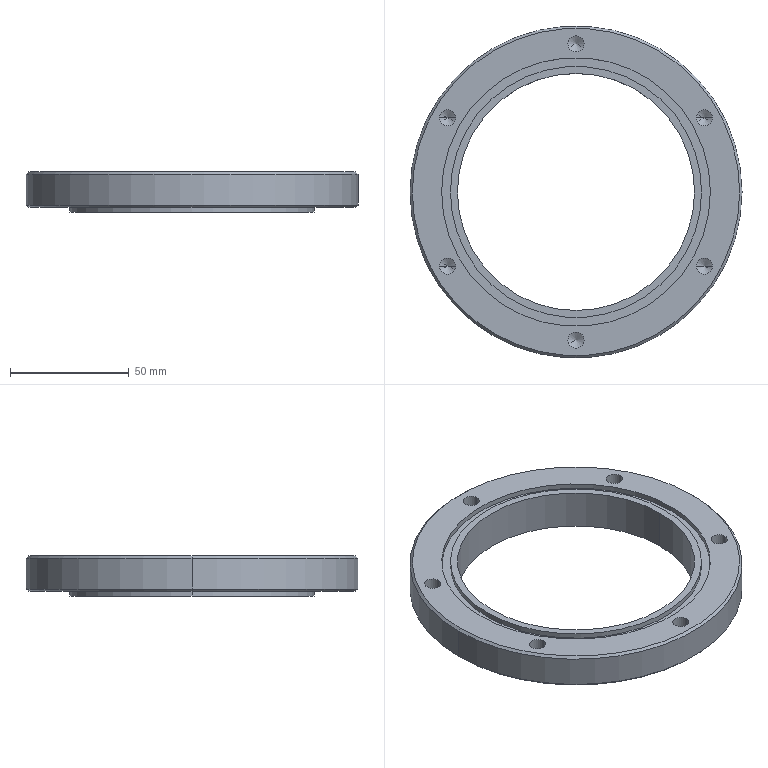Part | SolidWorks | features ICE 3, Chamfer 1, Extrusion 1, HoleWzd 1 | 1 solid | 43 faces | box 140 x 140 x 17 mm | volume 108486 mm3 | cylinder 22 | cone 16 | plane 5 | commonest cylinder face diameters 6.8 x12 100 x2 103 x2 105.9 x2 113.3 x2 140 x2
STEP:
#1=CARTESIAN_POINT('',(69.,0.,17.));
#2=VERTEX_POINT('',#1);
#3=CARTESIAN_POINT('',(-69.,0.,17.));
#4=VERTEX_POINT('',#3);
#5=CARTESIAN_POINT('',(0.,0.,17.));
#6=DIRECTION('',(0.,0.,1.));
#7=DIRECTION('',(1.,0.,0.));
#8=AXIS2_PLACEMENT_3D('',#5,#6,#7);
#9=CIRCLE('',#8,69.);
#10=EDGE_CURVE('',#2,#4,#9,.T.);
#11=ORIENTED_EDGE('',*,*,#10,.F.);
#12=CARTESIAN_POINT('',(70.,0.,16.));
#13=VERTEX_POINT('',#12);
#14=CARTESIAN_POINT('',(69.,0.,17.));
#15=DIRECTION('',(0.7071,0.,-0.7071));
#16=VECTOR('',#15,1000.);
#17=LINE('',#14,#16);
#18=EDGE_CURVE('',#2,#13,#17,.T.);
#19=ORIENTED_EDGE('',*,*,#18,.T.);
#20=CARTESIAN_POINT('',(-70.,0.,16.));
#21=VERTEX_POINT('',#20);
#22=CARTESIAN_POINT('',(0.,0.,16.));
#23=DIRECTION('',(0.,0.,-1.));
#24=DIRECTION('',(1.,0.,0.));
#25=AXIS2_PLACEMENT_3D('',#22,#23,#24);
#26=CIRCLE('',#25,70.);
#27=EDGE_CURVE('',#21,#13,#26,.T.);
#28=ORIENTED_EDGE('',*,*,#27,.F.);
#29=CARTESIAN_POINT('',(-69.,0.,17.));
#30=DIRECTION('',(-0.7071,0.,-0.7071));
#31=VECTOR('',#30,1000.);
#32=LINE('',#29,#31);
#33=EDGE_CURVE('',#4,#21,#32,.T.);
#34=ORIENTED_EDGE('',*,*,#33,.F.);
#35=EDGE_LOOP('',(#11,#19,#28,#34));
#36=FACE_OUTER_BOUND('',#35,.T.);
#37=CARTESIAN_POINT('',(0.,0.,17.));
#38=DIRECTION('',(0.,0.,-1.));
#39=DIRECTION('',(-1.,0.,0.));
#40=AXIS2_PLACEMENT_3D('',#37,#38,#39);
#41=CONICAL_SURFACE('',#40,69.,0.7854);
#42=ADVANCED_FACE('',(#36),#41,.T.);
#43=CARTESIAN_POINT('',(-69.,0.,2.));
#44=VERTEX_POINT('',#43);
#45=CARTESIAN_POINT('',(69.,0.,2.));
#46=VERTEX_POINT('',#45);
#47=CARTESIAN_POINT('',(0.,0.,2.));
#48=DIRECTION('',(0.,0.,-1.));
#49=DIRECTION('',(-1.,0.,0.));
#50=AXIS2_PLACEMENT_3D('',#47,#48,#49);
#51=CIRCLE('',#50,69.);
#52=EDGE_CURVE('',#44,#46,#51,.T.);
#53=ORIENTED_EDGE('',*,*,#52,.F.);
#54=CARTESIAN_POINT('',(-70.,0.,3.));
#55=VERTEX_POINT('',#54);
#56=CARTESIAN_POINT('',(-69.,0.,2.));
#57=DIRECTION('',(-0.7071,0.,0.7071));
#58=VECTOR('',#57,1000.);
#59=LINE('',#56,#58);
#60=EDGE_CURVE('',#44,#55,#59,.T.);
#61=ORIENTED_EDGE('',*,*,#60,.T.);
#62=CARTESIAN_POINT('',(70.,0.,3.));
#63=VERTEX_POINT('',#62);
#64=CARTESIAN_POINT('',(0.,0.,3.));
#65=DIRECTION('',(0.,0.,1.));
#66=DIRECTION('',(-1.,0.,0.));
#67=AXIS2_PLACEMENT_3D('',#64,#65,#66);
#68=CIRCLE('',#67,70.);
#69=EDGE_CURVE('',#63,#55,#68,.T.);
#70=ORIENTED_EDGE('',*,*,#69,.F.);
#71=CARTESIAN_POINT('',(69.,0.,2.));
#72=DIRECTION('',(0.7071,0.,0.7071));
#73=VECTOR('',#72,1000.);
#74=LINE('',#71,#73);
#75=EDGE_CURVE('',#46,#63,#74,.T.);
#76=ORIENTED_EDGE('',*,*,#75,.F.);
#77=EDGE_LOOP('',(#53,#61,#70,#76));
#78=FACE_OUTER_BOUND('',#77,.T.);
#79=CARTESIAN_POINT('',(0.,0.,2.));
#80=DIRECTION('',(0.,0.,1.));
#81=DIRECTION('',(1.,0.,0.));
#82=AXIS2_PLACEMENT_3D('',#79,#80,#81);
#83=CONICAL_SURFACE('',#82,69.,0.7854);
#84=ADVANCED_FACE('',(#78),#83,.T.);
#85=CARTESIAN_POINT('',(-3.4,62.5,7.));
#86=VERTEX_POINT('',#85);
#87=CARTESIAN_POINT('',(3.4,62.5,7.));
#88=VERTEX_POINT('',#87);
#89=CARTESIAN_POINT('',(0.,62.5,7.));
#90=DIRECTION('',(0.,0.,1.));
#91=DIRECTION('',(1.,0.,0.));
#92=AXIS2_PLACEMENT_3D('',#89,#90,#91);
#93=CIRCLE('',#92,3.4);
#94=EDGE_CURVE('',#86,#88,#93,.T.);
#95=ORIENTED_EDGE('',*,*,#94,.F.);
#96=CARTESIAN_POINT('',(-3.4,62.5,17.));
#97=VERTEX_POINT('',#96);
#98=CARTESIAN_POINT('',(-3.4,62.5,17.));
#99=DIRECTION('',(0.,0.,1.));
#100=VECTOR('',#99,1000.);
#101=LINE('',#98,#100);
#102=EDGE_CURVE('',#86,#97,#101,.T.);
#103=ORIENTED_EDGE('',*,*,#102,.T.);
#104=CARTESIAN_POINT('',(3.4,62.5,17.));
#105=VERTEX_POINT('',#104);
#106=CARTESIAN_POINT('',(0.,62.5,17.));
#107=DIRECTION('',(0.,0.,1.));
#108=DIRECTION('',(1.,0.,0.));
#109=AXIS2_PLACEMENT_3D('',#106,#107,#108);
#110=CIRCLE('',#109,3.4);
#111=EDGE_CURVE('',#97,#105,#110,.T.);
#112=ORIENTED_EDGE('',*,*,#111,.T.);
#113=CARTESIAN_POINT('',(3.4,62.5,17.));
#114=DIRECTION('',(0.,0.,1.));
#115=VECTOR('',#114,1000.);
#116=LINE('',#113,#115);
#117=EDGE_CURVE('',#88,#105,#116,.T.);
#118=ORIENTED_EDGE('',*,*,#117,.F.);
#119=EDGE_LOOP('',(#95,#103,#112,#118));
#120=FACE_OUTER_BOUND('',#119,.T.);
#121=CARTESIAN_POINT('',(0.,62.5,17.));
#122=DIRECTION('',(0.,0.,1.));
#123=DIRECTION('',(1.,0.,0.));
#124=AXIS2_PLACEMENT_3D('',#121,#122,#123);
#125=CYLINDRICAL_SURFACE('',#124,3.4);
#126=ADVANCED_FACE('',(#120),#125,.F.);
#127=CARTESIAN_POINT('',(0.,62.5,4.957));
#128=VERTEX_POINT('',#127);
#129=CARTESIAN_POINT('',(3.4,62.5,7.));
#130=DIRECTION('',(0.8572,0.,0.515));
#131=VECTOR('',#130,1000.);
#132=LINE('',#129,#131);
#133=EDGE_CURVE('',#128,#88,#132,.T.);
#134=ORIENTED_EDGE('',*,*,#133,.F.);
#135=CARTESIAN_POINT('',(-3.4,62.5,7.));
#136=DIRECTION('',(-0.8572,0.,0.515));
#137=VECTOR('',#136,1000.);
#138=LINE('',#135,#137);
#139=EDGE_CURVE('',#128,#86,#138,.T.);
#140=ORIENTED_EDGE('',*,*,#139,.T.);
#141=ORIENTED_EDGE('',*,*,#94,.T.);
#142=EDGE_LOOP('',(#134,#140,#141));
#143=FACE_OUTER_BOUND('',#142,.T.);
#144=CARTESIAN_POINT('',(0.,62.5,7.));
#145=DIRECTION('',(0.,0.,1.));
#146=DIRECTION('',(1.,0.,0.));
#147=AXIS2_PLACEMENT_3D('',#144,#145,#146);
#148=CONICAL_SURFACE('',#147,3.4,1.03);
#149=ADVANCED_FACE('',(#143),#148,.F.);
#150=CARTESIAN_POINT('',(50.727,31.25,7.));
#151=VERTEX_POINT('',#150);
#152=CARTESIAN_POINT('',(57.527,31.25,7.));
#153=VERTEX_POINT('',#152);
#154=CARTESIAN_POINT('',(54.127,31.25,7.));
#155=DIRECTION('',(0.,0.,1.));
#156=DIRECTION('',(1.,0.,0.));
#157=AXIS2_PLACEMENT_3D('',#154,#155,#156);
#158=CIRCLE('',#157,3.4);
#159=EDGE_CURVE('',#151,#153,#158,.T.);
#160=ORIENTED_EDGE('',*,*,#159,.F.);
#161=CARTESIAN_POINT('',(50.727,31.25,17.));
#162=VERTEX_POINT('',#161);
#163=CARTESIAN_POINT('',(50.727,31.25,17.));
#164=DIRECTION('',(0.,0.,1.));
#165=VECTOR('',#164,1000.);
#166=LINE('',#163,#165);
#167=EDGE_CURVE('',#151,#162,#166,.T.);
#168=ORIENTED_EDGE('',*,*,#167,.T.);
#169=CARTESIAN_POINT('',(57.527,31.25,17.));
#170=VERTEX_POINT('',#169);
#171=CARTESIAN_POINT('',(54.127,31.25,17.));
#172=DIRECTION('',(0.,0.,1.));
#173=DIRECTION('',(1.,0.,0.));
#174=AXIS2_PLACEMENT_3D('',#171,#172,#173);
#175=CIRCLE('',#174,3.4);
#176=EDGE_CURVE('',#162,#170,#175,.T.);
#177=ORIENTED_EDGE('',*,*,#176,.T.);
#178=CARTESIAN_POINT('',(57.527,31.25,17.));
#179=DIRECTION('',(0.,0.,1.));
#180=VECTOR('',#179,1000.);
#181=LINE('',#178,#180);
#182=EDGE_CURVE('',#153,#170,#181,.T.);
#183=ORIENTED_EDGE('',*,*,#182,.F.);
#184=EDGE_LOOP('',(#160,#168,#177,#183));
#185=FACE_OUTER_BOUND('',#184,.T.);
#186=CARTESIAN_POINT('',(54.127,31.25,17.));
#187=DIRECTION('',(0.,0.,1.));
#188=DIRECTION('',(1.,0.,0.));
#189=AXIS2_PLACEMENT_3D('',#186,#187,#188);
#190=CYLINDRICAL_SURFACE('',#189,3.4);
#191=ADVANCED_FACE('',(#185),#190,.F.);
#192=CARTESIAN_POINT('',(54.127,31.25,4.957));
#193=VERTEX_POINT('',#192);
#194=CARTESIAN_POINT('',(57.527,31.25,7.));
#195=DIRECTION('',(0.8572,0.,0.515));
#196=VECTOR('',#195,1000.);
#197=LINE('',#194,#196);
#198=EDGE_CURVE('',#193,#153,#197,.T.);
#199=ORIENTED_EDGE('',*,*,#198,.F.);
#200=CARTESIAN_POINT('',(50.727,31.25,7.));
#201=DIRECTION('',(-0.8572,0.,0.515));
#202=VECTOR('',#201,1000.);
#203=LINE('',#200,#202);
#204=EDGE_CURVE('',#193,#151,#203,.T.);
#205=ORIENTED_EDGE('',*,*,#204,.T.);
#206=ORIENTED_EDGE('',*,*,#159,.T.);
#207=EDGE_LOOP('',(#199,#205,#206));
#208=FACE_OUTER_BOUND('',#207,.T.);
#209=CARTESIAN_POINT('',(54.127,31.25,7.));
#210=DIRECTION('',(0.,0.,1.));
#211=DIRECTION('',(1.,0.,0.));
#212=AXIS2_PLACEMENT_3D('',#209,#210,#211);
#213=CONICAL_SURFACE('',#212,3.4,1.03);
#214=ADVANCED_FACE('',(#208),#213,.F.);
#215=CARTESIAN_POINT('',(50.727,-31.25,7.));
#216=VERTEX_POINT('',#215);
#217=CARTESIAN_POINT('',(57.527,-31.25,7.));
#218=VERTEX_POINT('',#217);
#219=CARTESIAN_POINT('',(54.127,-31.25,7.));
#220=DIRECTION('',(0.,0.,1.));
#221=DIRECTION('',(1.,0.,0.));
#222=AXIS2_PLACEMENT_3D('',#219,#220,#221);
#223=CIRCLE('',#222,3.4);
#224=EDGE_CURVE('',#216,#218,#223,.T.);
#225=ORIENTED_EDGE('',*,*,#224,.F.);
#226=CARTESIAN_POINT('',(50.727,-31.25,17.));
#227=VERTEX_POINT('',#226);
#228=CARTESIAN_POINT('',(50.727,-31.25,17.));
#229=DIRECTION('',(0.,0.,1.));
#230=VECTOR('',#229,1000.);
#231=LINE('',#228,#230);
#232=EDGE_CURVE('',#216,#227,#231,.T.);
#233=ORIENTED_EDGE('',*,*,#232,.T.);
#234=CARTESIAN_POINT('',(57.527,-31.25,17.));
#235=VERTEX_POINT('',#234);
#236=CARTESIAN_POINT('',(54.127,-31.25,17.));
#237=DIRECTION('',(0.,0.,1.));
#238=DIRECTION('',(1.,0.,0.));
#239=AXIS2_PLACEMENT_3D('',#236,#237,#238);
#240=CIRCLE('',#239,3.4);
#241=EDGE_CURVE('',#227,#235,#240,.T.);
#242=ORIENTED_EDGE('',*,*,#241,.T.);
#243=CARTESIAN_POINT('',(57.527,-31.25,17.));
#244=DIRECTION('',(0.,0.,1.));
#245=VECTOR('',#244,1000.);
#246=LINE('',#243,#245);
#247=EDGE_CURVE('',#218,#235,#246,.T.);
#248=ORIENTED_EDGE('',*,*,#247,.F.);
#249=EDGE_LOOP('',(#225,#233,#242,#248));
#250=FACE_OUTER_BOUND('',#249,.T.);
#251=CARTESIAN_POINT('',(54.127,-31.25,17.));
#252=DIRECTION('',(0.,0.,1.));
#253=DIRECTION('',(1.,0.,0.));
#254=AXIS2_PLACEMENT_3D('',#251,#252,#253);
#255=CYLINDRICAL_SURFACE('',#254,3.4);
#256=ADVANCED_FACE('',(#250),#255,.F.);
#257=CARTESIAN_POINT('',(54.127,-31.25,4.957));
#258=VERTEX_POINT('',#257);
#259=CARTESIAN_POINT('',(57.527,-31.25,7.));
#260=DIRECTION('',(0.8572,0.,0.515));
#261=VECTOR('',#260,1000.);
#262=LINE('',#259,#261);
#263=EDGE_CURVE('',#258,#218,#262,.T.);
#264=ORIENTED_EDGE('',*,*,#263,.F.);
#265=CARTESIAN_POINT('',(50.727,-31.25,7.));
#266=DIRECTION('',(-0.8572,0.,0.515));
#267=VECTOR('',#266,1000.);
#268=LINE('',#265,#267);
#269=EDGE_CURVE('',#258,#216,#268,.T.);
#270=ORIENTED_EDGE('',*,*,#269,.T.);
#271=ORIENTED_EDGE('',*,*,#224,.T.);
#272=EDGE_LOOP('',(#264,#270,#271));
#273=FACE_OUTER_BOUND('',#272,.T.);
#274=CARTESIAN_POINT('',(54.127,-31.25,7.));
#275=DIRECTION('',(0.,0.,1.));
#276=DIRECTION('',(1.,0.,0.));
#277=AXIS2_PLACEMENT_3D('',#274,#275,#276);
#278=CONICAL_SURFACE('',#277,3.4,1.03);
#279=ADVANCED_FACE('',(#273),#278,.F.);
#280=CARTESIAN_POINT('',(-3.4,-62.5,7.));
#281=VERTEX_POINT('',#280);
#282=CARTESIAN_POINT('',(3.4,-62.5,7.));
#283=VERTEX_POINT('',#282);
#284=CARTESIAN_POINT('',(0.,-62.5,7.));
#285=DIRECTION('',(0.,0.,1.));
#286=DIRECTION('',(1.,0.,0.));
#287=AXIS2_PLACEMENT_3D('',#284,#285,#286);
#288=CIRCLE('',#287,3.4);
#289=EDGE_CURVE('',#281,#283,#288,.T.);
#290=ORIENTED_EDGE('',*,*,#289,.F.);
#291=CARTESIAN_POINT('',(-3.4,-62.5,17.));
#292=VERTEX_POINT('',#291);
#293=CARTESIAN_POINT('',(-3.4,-62.5,17.));
#294=DIRECTION('',(0.,0.,1.));
#295=VECTOR('',#294,1000.);
#296=LINE('',#293,#295);
#297=EDGE_CURVE('',#281,#292,#296,.T.);
#298=ORIENTED_EDGE('',*,*,#297,.T.);
#299=CARTESIAN_POINT('',(3.4,-62.5,17.));
#300=VERTEX_POINT('',#299);
#301=CARTESIAN_POINT('',(0.,-62.5,17.));
#302=DIRECTION('',(0.,0.,1.));
#303=DIRECTION('',(1.,0.,0.));
#304=AXIS2_PLACEMENT_3D('',#301,#302,#303);
#305=CIRCLE('',#304,3.4);
#306=EDGE_CURVE('',#292,#300,#305,.T.);
#307=ORIENTED_EDGE('',*,*,#306,.T.);
#308=CARTESIAN_POINT('',(3.4,-62.5,17.));
#309=DIRECTION('',(0.,0.,1.));
#310=VECTOR('',#309,1000.);
#311=LINE('',#308,#310);
#312=EDGE_CURVE('',#283,#300,#311,.T.);
#313=ORIENTED_EDGE('',*,*,#312,.F.);
#314=EDGE_LOOP('',(#290,#298,#307,#313));
#315=FACE_OUTER_BOUND('',#314,.T.);
#316=CARTESIAN_POINT('',(0.,-62.5,17.));
#317=DIRECTION('',(0.,0.,1.));
#318=DIRECTION('',(1.,0.,0.));
#319=AXIS2_PLACEMENT_3D('',#316,#317,#318);
#320=CYLINDRICAL_SURFACE('',#319,3.4);
#321=ADVANCED_FACE('',(#315),#320,.F.);
#322=CARTESIAN_POINT('',(0.,-62.5,4.957));
#323=VERTEX_POINT('',#322);
#324=CARTESIAN_POINT('',(3.4,-62.5,7.));
#325=DIRECTION('',(0.8572,0.,0.515));
#326=VECTOR('',#325,1000.);
#327=LINE('',#324,#326);
#328=EDGE_CURVE('',#323,#283,#327,.T.);
#329=ORIENTED_EDGE('',*,*,#328,.F.);
#330=CARTESIAN_POINT('',(-3.4,-62.5,7.));
#331=DIRECTION('',(-0.8572,0.,0.515));
#332=VECTOR('',#331,1000.);
#333=LINE('',#330,#332);
#334=EDGE_CURVE('',#323,#281,#333,.T.);
#335=ORIENTED_EDGE('',*,*,#334,.T.);
#336=ORIENTED_EDGE('',*,*,#289,.T.);
#337=EDGE_LOOP('',(#329,#335,#336));
#338=FACE_OUTER_BOUND('',#337,.T.);
#339=CARTESIAN_POINT('',(0.,-62.5,7.));
#340=DIRECTION('',(0.,0.,1.));
#341=DIRECTION('',(1.,0.,0.));
#342=AXIS2_PLACEMENT_3D('',#339,#340,#341);
#343=CONICAL_SURFACE('',#342,3.4,1.03);
#344=ADVANCED_FACE('',(#338),#343,.F.);
#345=CARTESIAN_POINT('',(-57.527,-31.25,7.));
#346=VERTEX_POINT('',#345);
#347=CARTESIAN_POINT('',(-50.727,-31.25,7.));
#348=VERTEX_POINT('',#347);
#349=CARTESIAN_POINT('',(-54.127,-31.25,7.));
#350=DIRECTION('',(0.,0.,1.));
#351=DIRECTION('',(1.,0.,0.));
#352=AXIS2_PLACEMENT_3D('',#349,#350,#351);
#353=CIRCLE('',#352,3.4);
#354=EDGE_CURVE('',#346,#348,#353,.T.);
#355=ORIENTED_EDGE('',*,*,#354,.F.);
#356=CARTESIAN_POINT('',(-57.527,-31.25,17.));
#357=VERTEX_POINT('',#356);
#358=CARTESIAN_POINT('',(-57.527,-31.25,17.));
#359=DIRECTION('',(0.,0.,1.));
#360=VECTOR('',#359,1000.);
#361=LINE('',#358,#360);
#362=EDGE_CURVE('',#346,#357,#361,.T.);
#363=ORIENTED_EDGE('',*,*,#362,.T.);
#364=CARTESIAN_POINT('',(-50.727,-31.25,17.));
#365=VERTEX_POINT('',#364);
#366=CARTESIAN_POINT('',(-54.127,-31.25,17.));
#367=DIRECTION('',(0.,0.,1.));
#368=DIRECTION('',(1.,0.,0.));
#369=AXIS2_PLACEMENT_3D('',#366,#367,#368);
#370=CIRCLE('',#369,3.4);
#371=EDGE_CURVE('',#357,#365,#370,.T.);
#372=ORIENTED_EDGE('',*,*,#371,.T.);
#373=CARTESIAN_POINT('',(-50.727,-31.25,17.));
#374=DIRECTION('',(0.,0.,1.));
#375=VECTOR('',#374,1000.);
#376=LINE('',#373,#375);
#377=EDGE_CURVE('',#348,#365,#376,.T.);
#378=ORIENTED_EDGE('',*,*,#377,.F.);
#379=EDGE_LOOP('',(#355,#363,#372,#378));
#380=FACE_OUTER_BOUND('',#379,.T.);
#381=CARTESIAN_POINT('',(-54.127,-31.25,17.));
#382=DIRECTION('',(0.,0.,1.));
#383=DIRECTION('',(1.,0.,0.));
#384=AXIS2_PLACEMENT_3D('',#381,#382,#383);
#385=CYLINDRICAL_SURFACE('',#384,3.4);
#386=ADVANCED_FACE('',(#380),#385,.F.);
#387=CARTESIAN_POINT('',(-54.127,-31.25,4.957));
#388=VERTEX_POINT('',#387);
#389=CARTESIAN_POINT('',(-50.727,-31.25,7.));
#390=DIRECTION('',(0.8572,0.,0.515));
#391=VECTOR('',#390,1000.);
#392=LINE('',#389,#391);
#393=EDGE_CURVE('',#388,#348,#392,.T.);
#394=ORIENTED_EDGE('',*,*,#393,.F.);
#395=CARTESIAN_POINT('',(-57.527,-31.25,7.));
#396=DIRECTION('',(-0.8572,0.,0.515));
#397=VECTOR('',#396,1000.);
#398=LINE('',#395,#397);
#399=EDGE_CURVE('',#388,#346,#398,.T.);
#400=ORIENTED_EDGE('',*,*,#399,.T.);
#401=ORIENTED_EDGE('',*,*,#354,.T.);
#402=EDGE_LOOP('',(#394,#400,#401));
#403=FACE_OUTER_BOUND('',#402,.T.);
#404=CARTESIAN_POINT('',(-54.127,-31.25,7.));
#405=DIRECTION('',(0.,0.,1.));
#406=DIRECTION('',(1.,0.,0.));
#407=AXIS2_PLACEMENT_3D('',#404,#405,#406);
#408=CONICAL_SURFACE('',#407,3.4,1.03);
#409=ADVANCED_FACE('',(#403),#408,.F.);
#410=CARTESIAN_POINT('',(-57.527,31.25,7.));
#411=VERTEX_POINT('',#410);
#412=CARTESIAN_POINT('',(-50.727,31.25,7.));
#413=VERTEX_POINT('',#412);
#414=CARTESIAN_POINT('',(-54.127,31.25,7.));
#415=DIRECTION('',(0.,0.,1.));
#416=DIRECTION('',(1.,0.,0.));
#417=AXIS2_PLACEMENT_3D('',#414,#415,#416);
#418=CIRCLE('',#417,3.4);
#419=EDGE_CURVE('',#411,#413,#418,.T.);
#420=ORIENTED_EDGE('',*,*,#419,.F.);
#421=CARTESIAN_POINT('',(-57.527,31.25,17.));
#422=VERTEX_POINT('',#421);
#423=CARTESIAN_POINT('',(-57.527,31.25,17.));
#424=DIRECTION('',(0.,0.,1.));
#425=VECTOR('',#424,1000.);
#426=LINE('',#423,#425);
#427=EDGE_CURVE('',#411,#422,#426,.T.);
#428=ORIENTED_EDGE('',*,*,#427,.T.);
#429=CARTESIAN_POINT('',(-50.727,31.25,17.));
#430=VERTEX_POINT('',#429);
#431=CARTESIAN_POINT('',(-54.127,31.25,17.));
#432=DIRECTION('',(0.,0.,1.));
#433=DIRECTION('',(1.,0.,0.));
#434=AXIS2_PLACEMENT_3D('',#431,#432,#433);
#435=CIRCLE('',#434,3.4);
#436=EDGE_CURVE('',#422,#430,#435,.T.);
#437=ORIENTED_EDGE('',*,*,#436,.T.);
#438=CARTESIAN_POINT('',(-50.727,31.25,17.));
#439=DIRECTION('',(0.,0.,1.));
#440=VECTOR('',#439,1000.);
#441=LINE('',#438,#440);
#442=EDGE_CURVE('',#413,#430,#441,.T.);
#443=ORIENTED_EDGE('',*,*,#442,.F.);
#444=EDGE_LOOP('',(#420,#428,#437,#443));
#445=FACE_OUTER_BOUND('',#444,.T.);
#446=CARTESIAN_POINT('',(-54.127,31.25,17.));
#447=DIRECTION('',(0.,0.,1.));
#448=DIRECTION('',(1.,0.,0.));
#449=AXIS2_PLACEMENT_3D('',#446,#447,#448);
#450=CYLINDRICAL_SURFACE('',#449,3.4);
#451=ADVANCED_FACE('',(#445),#450,.F.);
#452=CARTESIAN_POINT('',(-54.127,31.25,4.957));
#453=VERTEX_POINT('',#452);
#454=CARTESIAN_POINT('',(-50.727,31.25,7.));
#455=DIRECTION('',(0.8572,0.,0.515));
#456=VECTOR('',#455,1000.);
#457=LINE('',#454,#456);
#458=EDGE_CURVE('',#453,#413,#457,.T.);
#459=ORIENTED_EDGE('',*,*,#458,.F.);
#460=CARTESIAN_POINT('',(-57.527,31.25,7.));
#461=DIRECTION('',(-0.8572,0.,0.515));
#462=VECTOR('',#461,1000.);
#463=LINE('',#460,#462);
#464=EDGE_CURVE('',#453,#411,#463,.T.);
#465=ORIENTED_EDGE('',*,*,#464,.T.);
#466=ORIENTED_EDGE('',*,*,#419,.T.);
#467=EDGE_LOOP('',(#459,#465,#466));
#468=FACE_OUTER_BOUND('',#467,.T.);
#469=CARTESIAN_POINT('',(-54.127,31.25,7.));
#470=DIRECTION('',(0.,0.,1.));
#471=DIRECTION('',(1.,0.,0.));
#472=AXIS2_PLACEMENT_3D('',#469,#470,#471);
#473=CONICAL_SURFACE('',#472,3.4,1.03);
#474=ADVANCED_FACE('',(#468),#473,.F.);
#475=CARTESIAN_POINT('',(-51.5,0.,2.));
#476=VERTEX_POINT('',#475);
#477=CARTESIAN_POINT('',(51.5,0.,2.));
#478=VERTEX_POINT('',#477);
#479=CARTESIAN_POINT('',(0.,0.,2.));
#480=DIRECTION('',(0.,0.,-1.));
#481=DIRECTION('',(-1.,0.,0.));
#482=AXIS2_PLACEMENT_3D('',#479,#480,#481);
#483=CIRCLE('',#482,51.5);
#484=EDGE_CURVE('',#476,#478,#483,.T.);
#485=ORIENTED_EDGE('',*,*,#484,.T.);
#486=CARTESIAN_POINT('',(51.5,0.,0.));
#487=VERTEX_POINT('',#486);
#488=CARTESIAN_POINT('',(51.5,0.,2.));
#489=DIRECTION('',(0.,0.,-1.));
#490=VECTOR('',#489,1000.);
#491=LINE('',#488,#490);
#492=EDGE_CURVE('',#478,#487,#491,.T.);
#493=ORIENTED_EDGE('',*,*,#492,.T.);
#494=CARTESIAN_POINT('',(-51.5,0.,0.));
#495=VERTEX_POINT('',#494);
#496=CARTESIAN_POINT('',(0.,0.,0.));
#497=DIRECTION('',(0.,0.,-1.));
#498=DIRECTION('',(-1.,0.,0.));
#499=AXIS2_PLACEMENT_3D('',#496,#497,#498);
#500=CIRCLE('',#499,51.5);
#501=EDGE_CURVE('',#495,#487,#500,.T.);
#502=ORIENTED_EDGE('',*,*,#501,.F.);
#503=CARTESIAN_POINT('',(-51.5,0.,2.));
#504=DIRECTION('',(0.,0.,-1.));
#505=VECTOR('',#504,1000.);
#506=LINE('',#503,#505);
#507=EDGE_CURVE('',#476,#495,#506,.T.);
#508=ORIENTED_EDGE('',*,*,#507,.F.);
#509=EDGE_LOOP('',(#485,#493,#502,#508));
#510=FACE_OUTER_BOUND('',#509,.T.);
#511=CARTESIAN_POINT('',(0.,0.,2.));
#512=DIRECTION('',(0.,0.,-1.));
#513=DIRECTION('',(-1.,0.,0.));
#514=AXIS2_PLACEMENT_3D('',#511,#512,#513);
#515=CYLINDRICAL_SURFACE('',#514,51.5);
#516=ADVANCED_FACE('',(#510),#515,.T.);
#517=CARTESIAN_POINT('',(52.95,0.,14.8));
#518=VERTEX_POINT('',#517);
#519=CARTESIAN_POINT('',(-52.95,0.,14.8));
#520=VERTEX_POINT('',#519);
#521=CARTESIAN_POINT('',(0.,0.,14.8));
#522=DIRECTION('',(0.,0.,1.));
#523=DIRECTION('',(1.,0.,0.));
#524=AXIS2_PLACEMENT_3D('',#521,#522,#523);
#525=CIRCLE('',#524,52.95);
#526=EDGE_CURVE('',#518,#520,#525,.T.);
#527=ORIENTED_EDGE('',*,*,#526,.T.);
#528=CARTESIAN_POINT('',(-52.95,0.,17.));
#529=VERTEX_POINT('',#528);
#530=CARTESIAN_POINT('',(-52.95,0.,14.8));
#531=DIRECTION('',(0.,0.,1.));
#532=VECTOR('',#531,1000.);
#533=LINE('',#530,#532);
#534=EDGE_CURVE('',#520,#529,#533,.T.);
#535=ORIENTED_EDGE('',*,*,#534,.T.);
#536=CARTESIAN_POINT('',(52.95,0.,17.));
#537=VERTEX_POINT('',#536);
#538=CARTESIAN_POINT('',(0.,0.,17.));
#539=DIRECTION('',(0.,0.,1.));
#540=DIRECTION('',(1.,0.,0.));
#541=AXIS2_PLACEMENT_3D('',#538,#539,#540);
#542=CIRCLE('',#541,52.95);
#543=EDGE_CURVE('',#537,#529,#542,.T.);
#544=ORIENTED_EDGE('',*,*,#543,.F.);
#545=CARTESIAN_POINT('',(52.95,0.,14.8));
#546=DIRECTION('',(0.,0.,1.));
#547=VECTOR('',#546,1000.);
#548=LINE('',#545,#547);
#549=EDGE_CURVE('',#518,#537,#548,.T.);
#550=ORIENTED_EDGE('',*,*,#549,.F.);
#551=EDGE_LOOP('',(#527,#535,#544,#550));
#552=FACE_OUTER_BOUND('',#551,.T.);
#553=CARTESIAN_POINT('',(0.,0.,14.8));
#554=DIRECTION('',(0.,0.,1.));
#555=DIRECTION('',(1.,0.,0.));
#556=AXIS2_PLACEMENT_3D('',#553,#554,#555);
#557=CYLINDRICAL_SURFACE('',#556,52.95);
#558=ADVANCED_FACE('',(#552),#557,.T.);
#559=CARTESIAN_POINT('',(-56.65,0.,14.8));
#560=VERTEX_POINT('',#559);
#561=CARTESIAN_POINT('',(56.65,0.,14.8));
#562=VERTEX_POINT('',#561);
#563=CARTESIAN_POINT('',(0.,0.,14.8));
#564=DIRECTION('',(0.,0.,1.));
#565=DIRECTION('',(1.,0.,0.));
#566=AXIS2_PLACEMENT_3D('',#563,#564,#565);
#567=CIRCLE('',#566,56.65);
#568=EDGE_CURVE('',#560,#562,#567,.T.);
#569=ORIENTED_EDGE('',*,*,#568,.F.);
#570=CARTESIAN_POINT('',(-56.65,0.,17.));
#571=VERTEX_POINT('',#570);
#572=CARTESIAN_POINT('',(-56.65,0.,14.8));
#573=DIRECTION('',(0.,0.,1.));
#574=VECTOR('',#573,1000.);
#575=LINE('',#572,#574);
#576=EDGE_CURVE('',#560,#571,#575,.T.);
#577=ORIENTED_EDGE('',*,*,#576,.T.);
#578=CARTESIAN_POINT('',(56.65,0.,17.));
#579=VERTEX_POINT('',#578);
#580=CARTESIAN_POINT('',(0.,0.,17.));
#581=DIRECTION('',(0.,0.,1.));
#582=DIRECTION('',(1.,0.,0.));
#583=AXIS2_PLACEMENT_3D('',#580,#581,#582);
#584=CIRCLE('',#583,56.65);
#585=EDGE_CURVE('',#571,#579,#584,.T.);
#586=ORIENTED_EDGE('',*,*,#585,.T.);
#587=CARTESIAN_POINT('',(56.65,0.,14.8));
#588=DIRECTION('',(0.,0.,1.));
#589=VECTOR('',#588,1000.);
#590=LINE('',#587,#589);
#591=EDGE_CURVE('',#562,#579,#590,.T.);
#592=ORIENTED_EDGE('',*,*,#591,.F.);
#593=EDGE_LOOP('',(#569,#577,#586,#592));
#594=FACE_OUTER_BOUND('',#593,.T.);
#595=CARTESIAN_POINT('',(0.,0.,14.8));
#596=DIRECTION('',(0.,0.,1.));
#597=DIRECTION('',(1.,0.,0.));
#598=AXIS2_PLACEMENT_3D('',#595,#596,#597);
#599=CYLINDRICAL_SURFACE('',#598,56.65);
#600=ADVANCED_FACE('',(#594),#599,.F.);
#601=CARTESIAN_POINT('',(-50.,0.,17.));
#602=VERTEX_POINT('',#601);
#603=CARTESIAN_POINT('',(50.,0.,17.));
#604=VERTEX_POINT('',#603);
#605=CARTESIAN_POINT('',(0.,0.,17.));
#606=DIRECTION('',(0.,0.,1.));
#607=DIRECTION('',(1.,0.,0.));
#608=AXIS2_PLACEMENT_3D('',#605,#606,#607);
#609=CIRCLE('',#608,50.);
#610=EDGE_CURVE('',#602,#604,#609,.T.);
#611=ORIENTED_EDGE('',*,*,#610,.T.);
#612=CARTESIAN_POINT('',(50.,0.,0.));
#613=VERTEX_POINT('',#612);
#614=CARTESIAN_POINT('',(50.,0.,17.));
#615=DIRECTION('',(0.,0.,-1.));
#616=VECTOR('',#615,1000.);
#617=LINE('',#614,#616);
#618=EDGE_CURVE('',#604,#613,#617,.T.);
#619=ORIENTED_EDGE('',*,*,#618,.T.);
#620=CARTESIAN_POINT('',(-50.,0.,0.));
#621=VERTEX_POINT('',#620);
#622=CARTESIAN_POINT('',(0.,0.,0.));
#623=DIRECTION('',(0.,0.,1.));
#624=DIRECTION('',(1.,0.,0.));
#625=AXIS2_PLACEMENT_3D('',#622,#623,#624);
#626=CIRCLE('',#625,50.);
#627=EDGE_CURVE('',#621,#613,#626,.T.);
#628=ORIENTED_EDGE('',*,*,#627,.F.);
#629=CARTESIAN_POINT('',(-50.,0.,17.));
#630=DIRECTION('',(0.,0.,-1.));
#631=VECTOR('',#630,1000.);
#632=LINE('',#629,#631);
#633=EDGE_CURVE('',#602,#621,#632,.T.);
#634=ORIENTED_EDGE('',*,*,#633,.F.);
#635=EDGE_LOOP('',(#611,#619,#628,#634));
#636=FACE_OUTER_BOUND('',#635,.T.);
#637=CARTESIAN_POINT('',(0.,0.,17.));
#638=DIRECTION('',(0.,0.,-1.));
#639=DIRECTION('',(-1.,0.,0.));
#640=AXIS2_PLACEMENT_3D('',#637,#638,#639);
#641=CYLINDRICAL_SURFACE('',#640,50.);
#642=ADVANCED_FACE('',(#636),#641,.F.);
#643=ORIENTED_EDGE('',*,*,#27,.T.);
#644=CARTESIAN_POINT('',(70.,0.,17.));
#645=DIRECTION('',(0.,0.,-1.));
#646=VECTOR('',#645,1000.);
#647=LINE('',#644,#646);
#648=EDGE_CURVE('',#13,#63,#647,.T.);
#649=ORIENTED_EDGE('',*,*,#648,.T.);
#650=ORIENTED_EDGE('',*,*,#69,.T.);
#651=CARTESIAN_POINT('',(-70.,0.,17.));
#652=DIRECTION('',(0.,0.,-1.));
#653=VECTOR('',#652,1000.);
#654=LINE('',#651,#653);
#655=EDGE_CURVE('',#21,#55,#654,.T.);
#656=ORIENTED_EDGE('',*,*,#655,.F.);
#657=EDGE_LOOP('',(#643,#649,#650,#656));
#658=FACE_OUTER_BOUND('',#657,.T.);
#659=CARTESIAN_POINT('',(0.,0.,17.));
#660=DIRECTION('',(0.,0.,-1.));
#661=DIRECTION('',(-1.,0.,0.));
#662=AXIS2_PLACEMENT_3D('',#659,#660,#661);
#663=CYLINDRICAL_SURFACE('',#662,70.);
#664=ADVANCED_FACE('',(#658),#663,.T.);
#665=ORIENTED_EDGE('',*,*,#627,.T.);
#666=CARTESIAN_POINT('',(0.,0.,0.));
#667=DIRECTION('',(0.,0.,1.));
#668=DIRECTION('',(1.,0.,0.));
#669=AXIS2_PLACEMENT_3D('',#666,#667,#668);
#670=CIRCLE('',#669,50.);
#671=EDGE_CURVE('',#613,#621,#670,.T.);
#672=ORIENTED_EDGE('',*,*,#671,.T.);
#673=EDGE_LOOP('',(#665,#672));
#674=FACE_BOUND('',#673,.T.);
#675=ORIENTED_EDGE('',*,*,#501,.T.);
#676=CARTESIAN_POINT('',(0.,0.,0.));
#677=DIRECTION('',(0.,0.,-1.));
#678=DIRECTION('',(-1.,0.,0.));
#679=AXIS2_PLACEMENT_3D('',#676,#677,#678);
#680=CIRCLE('',#679,51.5);
#681=EDGE_CURVE('',#487,#495,#680,.T.);
#682=ORIENTED_EDGE('',*,*,#681,.T.);
#683=EDGE_LOOP('',(#675,#682));
#684=FACE_OUTER_BOUND('',#683,.T.);
#685=CARTESIAN_POINT('',(0.,0.,0.));
#686=DIRECTION('',(0.,0.,1.));
#687=DIRECTION('',(1.,0.,0.));
#688=AXIS2_PLACEMENT_3D('',#685,#686,#687);
#689=PLANE('',#688);
#690=ADVANCED_FACE('',(#674,#684),#689,.F.);
#691=ORIENTED_EDGE('',*,*,#648,.F.);
#692=CARTESIAN_POINT('',(0.,0.,16.));
#693=DIRECTION('',(0.,0.,-1.));
#694=DIRECTION('',(1.,0.,0.));
#695=AXIS2_PLACEMENT_3D('',#692,#693,#694);
#696=CIRCLE('',#695,70.);
#697=EDGE_CURVE('',#13,#21,#696,.T.);
#698=ORIENTED_EDGE('',*,*,#697,.T.);
#699=ORIENTED_EDGE('',*,*,#655,.T.);
#700=CARTESIAN_POINT('',(0.,0.,3.));
#701=DIRECTION('',(0.,0.,1.));
#702=DIRECTION('',(-1.,0.,0.));
#703=AXIS2_PLACEMENT_3D('',#700,#701,#702);
#704=CIRCLE('',#703,70.);
#705=EDGE_CURVE('',#55,#63,#704,.T.);
#706=ORIENTED_EDGE('',*,*,#705,.T.);
#707=EDGE_LOOP('',(#691,#698,#699,#706));
#708=FACE_OUTER_BOUND('',#707,.T.);
#709=CARTESIAN_POINT('',(0.,0.,17.));
#710=DIRECTION('',(0.,0.,-1.));
#711=DIRECTION('',(-1.,0.,0.));
#712=AXIS2_PLACEMENT_3D('',#709,#710,#711);
#713=CYLINDRICAL_SURFACE('',#712,70.);
#714=ADVANCED_FACE('',(#708),#713,.T.);
#715=ORIENTED_EDGE('',*,*,#610,.F.);
#716=CARTESIAN_POINT('',(0.,0.,17.));
#717=DIRECTION('',(0.,0.,1.));
#718=DIRECTION('',(1.,0.,0.));
#719=AXIS2_PLACEMENT_3D('',#716,#717,#718);
#720=CIRCLE('',#719,50.);
#721=EDGE_CURVE('',#604,#602,#720,.T.);
#722=ORIENTED_EDGE('',*,*,#721,.F.);
#723=EDGE_LOOP('',(#715,#722));
#724=FACE_BOUND('',#723,.T.);
#725=ORIENTED_EDGE('',*,*,#543,.T.);
#726=CARTESIAN_POINT('',(0.,0.,17.));
#727=DIRECTION('',(0.,0.,1.));
#728=DIRECTION('',(1.,0.,0.));
#729=AXIS2_PLACEMENT_3D('',#726,#727,#728);
#730=CIRCLE('',#729,52.95);
#731=EDGE_CURVE('',#529,#537,#730,.T.);
#732=ORIENTED_EDGE('',*,*,#731,.T.);
#733=EDGE_LOOP('',(#725,#732));
#734=FACE_OUTER_BOUND('',#733,.T.);
#735=CARTESIAN_POINT('',(0.,0.,17.));
#736=DIRECTION('',(0.,0.,1.));
#737=DIRECTION('',(1.,0.,0.));
#738=AXIS2_PLACEMENT_3D('',#735,#736,#737);
#739=PLANE('',#738);
#740=ADVANCED_FACE('',(#724,#734),#739,.T.);
#741=CARTESIAN_POINT('',(0.,0.,17.));
#742=DIRECTION('',(0.,0.,1.));
#743=DIRECTION('',(1.,0.,0.));
#744=AXIS2_PLACEMENT_3D('',#741,#742,#743);
#745=CIRCLE('',#744,69.);
#746=EDGE_CURVE('',#4,#2,#745,.T.);
#747=ORIENTED_EDGE('',*,*,#746,.T.);
#748=ORIENTED_EDGE('',*,*,#10,.T.);
#749=EDGE_LOOP('',(#747,#748));
#750=FACE_OUTER_BOUND('',#749,.T.);
#751=CARTESIAN_POINT('',(0.,62.5,17.));
#752=DIRECTION('',(0.,0.,1.));
#753=DIRECTION('',(1.,0.,0.));
#754=AXIS2_PLACEMENT_3D('',#751,#752,#753);
#755=CIRCLE('',#754,3.4);
#756=EDGE_CURVE('',#105,#97,#755,.T.);
#757=ORIENTED_EDGE('',*,*,#756,.F.);
#758=ORIENTED_EDGE('',*,*,#111,.F.);
#759=EDGE_LOOP('',(#757,#758));
#760=FACE_BOUND('',#759,.T.);
#761=CARTESIAN_POINT('',(54.127,31.25,17.));
#762=DIRECTION('',(0.,0.,1.));
#763=DIRECTION('',(1.,0.,0.));
#764=AXIS2_PLACEMENT_3D('',#761,#762,#763);
#765=CIRCLE('',#764,3.4);
#766=EDGE_CURVE('',#170,#162,#765,.T.);
#767=ORIENTED_EDGE('',*,*,#766,.F.);
#768=ORIENTED_EDGE('',*,*,#176,.F.);
#769=EDGE_LOOP('',(#767,#768));
#770=FACE_BOUND('',#769,.T.);
#771=CARTESIAN_POINT('',(54.127,-31.25,17.));
#772=DIRECTION('',(0.,0.,1.));
#773=DIRECTION('',(1.,0.,0.));
#774=AXIS2_PLACEMENT_3D('',#771,#772,#773);
#775=CIRCLE('',#774,3.4);
#776=EDGE_CURVE('',#235,#227,#775,.T.);
#777=ORIENTED_EDGE('',*,*,#776,.F.);
#778=ORIENTED_EDGE('',*,*,#241,.F.);
#779=EDGE_LOOP('',(#777,#778));
#780=FACE_BOUND('',#779,.T.);
#781=CARTESIAN_POINT('',(0.,-62.5,17.));
#782=DIRECTION('',(0.,0.,1.));
#783=DIRECTION('',(1.,0.,0.));
#784=AXIS2_PLACEMENT_3D('',#781,#782,#783);
#785=CIRCLE('',#784,3.4);
#786=EDGE_CURVE('',#300,#292,#785,.T.);
#787=ORIENTED_EDGE('',*,*,#786,.F.);
#788=ORIENTED_EDGE('',*,*,#306,.F.);
#789=EDGE_LOOP('',(#787,#788));
#790=FACE_BOUND('',#789,.T.);
#791=CARTESIAN_POINT('',(-54.127,-31.25,17.));
#792=DIRECTION('',(0.,0.,1.));
#793=DIRECTION('',(1.,0.,0.));
#794=AXIS2_PLACEMENT_3D('',#791,#792,#793);
#795=CIRCLE('',#794,3.4);
#796=EDGE_CURVE('',#365,#357,#795,.T.);
#797=ORIENTED_EDGE('',*,*,#796,.F.);
#798=ORIENTED_EDGE('',*,*,#371,.F.);
#799=EDGE_LOOP('',(#797,#798));
#800=FACE_BOUND('',#799,.T.);
#801=CARTESIAN_POINT('',(-54.127,31.25,17.));
#802=DIRECTION('',(0.,0.,1.));
#803=DIRECTION('',(1.,0.,0.));
#804=AXIS2_PLACEMENT_3D('',#801,#802,#803);
#805=CIRCLE('',#804,3.4);
#806=EDGE_CURVE('',#430,#422,#805,.T.);
#807=ORIENTED_EDGE('',*,*,#806,.F.);
#808=ORIENTED_EDGE('',*,*,#436,.F.);
#809=EDGE_LOOP('',(#807,#808));
#810=FACE_BOUND('',#809,.T.);
#811=CARTESIAN_POINT('',(0.,0.,17.));
#812=DIRECTION('',(0.,0.,1.));
#813=DIRECTION('',(1.,0.,0.));
#814=AXIS2_PLACEMENT_3D('',#811,#812,#813);
#815=CIRCLE('',#814,56.65);
#816=EDGE_CURVE('',#579,#571,#815,.T.);
#817=ORIENTED_EDGE('',*,*,#816,.F.);
#818=ORIENTED_EDGE('',*,*,#585,.F.);
#819=EDGE_LOOP('',(#817,#818));
#820=FACE_BOUND('',#819,.T.);
#821=CARTESIAN_POINT('',(0.,0.,17.));
#822=DIRECTION('',(0.,0.,1.));
#823=DIRECTION('',(1.,0.,0.));
#824=AXIS2_PLACEMENT_3D('',#821,#822,#823);
#825=PLANE('',#824);
#826=ADVANCED_FACE('',(#750,#760,#770,#780,#790,#800,#810,#820),#825,.T.);
#827=ORIENTED_EDGE('',*,*,#618,.F.);
#828=ORIENTED_EDGE('',*,*,#721,.T.);
#829=ORIENTED_EDGE('',*,*,#633,.T.);
#830=ORIENTED_EDGE('',*,*,#671,.F.);
#831=EDGE_LOOP('',(#827,#828,#829,#830));
#832=FACE_OUTER_BOUND('',#831,.T.);
#833=CARTESIAN_POINT('',(0.,0.,17.));
#834=DIRECTION('',(0.,0.,-1.));
#835=DIRECTION('',(-1.,0.,0.));
#836=AXIS2_PLACEMENT_3D('',#833,#834,#835);
#837=CYLINDRICAL_SURFACE('',#836,50.);
#838=ADVANCED_FACE('',(#832),#837,.F.);
#839=ORIENTED_EDGE('',*,*,#576,.F.);
#840=CARTESIAN_POINT('',(0.,0.,14.8));
#841=DIRECTION('',(0.,0.,1.));
#842=DIRECTION('',(1.,0.,0.));
#843=AXIS2_PLACEMENT_3D('',#840,#841,#842);
#844=CIRCLE('',#843,56.65);
#845=EDGE_CURVE('',#562,#560,#844,.T.);
#846=ORIENTED_EDGE('',*,*,#845,.F.);
#847=ORIENTED_EDGE('',*,*,#591,.T.);
#848=ORIENTED_EDGE('',*,*,#816,.T.);
#849=EDGE_LOOP('',(#839,#846,#847,#848));
#850=FACE_OUTER_BOUND('',#849,.T.);
#851=CARTESIAN_POINT('',(0.,0.,14.8));
#852=DIRECTION('',(0.,0.,1.));
#853=DIRECTION('',(1.,0.,0.));
#854=AXIS2_PLACEMENT_3D('',#851,#852,#853);
#855=CYLINDRICAL_SURFACE('',#854,56.65);
#856=ADVANCED_FACE('',(#850),#855,.F.);
#857=ORIENTED_EDGE('',*,*,#526,.F.);
#858=CARTESIAN_POINT('',(0.,0.,14.8));
#859=DIRECTION('',(0.,0.,1.));
#860=DIRECTION('',(1.,0.,0.));
#861=AXIS2_PLACEMENT_3D('',#858,#859,#860);
#862=CIRCLE('',#861,52.95);
#863=EDGE_CURVE('',#520,#518,#862,.T.);
#864=ORIENTED_EDGE('',*,*,#863,.F.);
#865=EDGE_LOOP('',(#857,#864));
#866=FACE_BOUND('',#865,.T.);
#867=ORIENTED_EDGE('',*,*,#845,.T.);
#868=ORIENTED_EDGE('',*,*,#568,.T.);
#869=EDGE_LOOP('',(#867,#868));
#870=FACE_OUTER_BOUND('',#869,.T.);
#871=CARTESIAN_POINT('',(0.,0.,14.8));
#872=DIRECTION('',(0.,0.,1.));
#873=DIRECTION('',(1.,0.,0.));
#874=AXIS2_PLACEMENT_3D('',#871,#872,#873);
#875=PLANE('',#874);
#876=ADVANCED_FACE('',(#866,#870),#875,.T.);
#877=ORIENTED_EDGE('',*,*,#534,.F.);
#878=ORIENTED_EDGE('',*,*,#863,.T.);
#879=ORIENTED_EDGE('',*,*,#549,.T.);
#880=ORIENTED_EDGE('',*,*,#731,.F.);
#881=EDGE_LOOP('',(#877,#878,#879,#880));
#882=FACE_OUTER_BOUND('',#881,.T.);
#883=CARTESIAN_POINT('',(0.,0.,14.8));
#884=DIRECTION('',(0.,0.,1.));
#885=DIRECTION('',(1.,0.,0.));
#886=AXIS2_PLACEMENT_3D('',#883,#884,#885);
#887=CYLINDRICAL_SURFACE('',#886,52.95);
#888=ADVANCED_FACE('',(#882),#887,.T.);
#889=CARTESIAN_POINT('',(0.,0.,2.));
#890=DIRECTION('',(0.,0.,-1.));
#891=DIRECTION('',(-1.,0.,0.));
#892=AXIS2_PLACEMENT_3D('',#889,#890,#891);
#893=CIRCLE('',#892,69.);
#894=EDGE_CURVE('',#46,#44,#893,.T.);
#895=ORIENTED_EDGE('',*,*,#894,.T.);
#896=ORIENTED_EDGE('',*,*,#52,.T.);
#897=EDGE_LOOP('',(#895,#896));
#898=FACE_OUTER_BOUND('',#897,.T.);
#899=ORIENTED_EDGE('',*,*,#484,.F.);
#900=CARTESIAN_POINT('',(0.,0.,2.));
#901=DIRECTION('',(0.,0.,-1.));
#902=DIRECTION('',(-1.,0.,0.));
#903=AXIS2_PLACEMENT_3D('',#900,#901,#902);
#904=CIRCLE('',#903,51.5);
#905=EDGE_CURVE('',#478,#476,#904,.T.);
#906=ORIENTED_EDGE('',*,*,#905,.F.);
#907=EDGE_LOOP('',(#899,#906));
#908=FACE_BOUND('',#907,.T.);
#909=CARTESIAN_POINT('',(0.,0.,2.));
#910=DIRECTION('',(0.,0.,-1.));
#911=DIRECTION('',(-1.,0.,0.));
#912=AXIS2_PLACEMENT_3D('',#909,#910,#911);
#913=PLANE('',#912);
#914=ADVANCED_FACE('',(#898,#908),#913,.T.);
#915=ORIENTED_EDGE('',*,*,#492,.F.);
#916=ORIENTED_EDGE('',*,*,#905,.T.);
#917=ORIENTED_EDGE('',*,*,#507,.T.);
#918=ORIENTED_EDGE('',*,*,#681,.F.);
#919=EDGE_LOOP('',(#915,#916,#917,#918));
#920=FACE_OUTER_BOUND('',#919,.T.);
#921=CARTESIAN_POINT('',(0.,0.,2.));
#922=DIRECTION('',(0.,0.,-1.));
#923=DIRECTION('',(-1.,0.,0.));
#924=AXIS2_PLACEMENT_3D('',#921,#922,#923);
#925=CYLINDRICAL_SURFACE('',#924,51.5);
#926=ADVANCED_FACE('',(#920),#925,.T.);
#927=ORIENTED_EDGE('',*,*,#464,.F.);
#928=ORIENTED_EDGE('',*,*,#458,.T.);
#929=CARTESIAN_POINT('',(-54.127,31.25,7.));
#930=DIRECTION('',(0.,0.,1.));
#931=DIRECTION('',(1.,0.,0.));
#932=AXIS2_PLACEMENT_3D('',#929,#930,#931);
#933=CIRCLE('',#932,3.4);
#934=EDGE_CURVE('',#413,#411,#933,.T.);
#935=ORIENTED_EDGE('',*,*,#934,.T.);
#936=EDGE_LOOP('',(#927,#928,#935));
#937=FACE_OUTER_BOUND('',#936,.T.);
#938=CARTESIAN_POINT('',(-54.127,31.25,7.));
#939=DIRECTION('',(0.,0.,1.));
#940=DIRECTION('',(1.,0.,0.));
#941=AXIS2_PLACEMENT_3D('',#938,#939,#940);
#942=CONICAL_SURFACE('',#941,3.4,1.03);
#943=ADVANCED_FACE('',(#937),#942,.F.);
#944=ORIENTED_EDGE('',*,*,#427,.F.);
#945=ORIENTED_EDGE('',*,*,#934,.F.);
#946=ORIENTED_EDGE('',*,*,#442,.T.);
#947=ORIENTED_EDGE('',*,*,#806,.T.);
#948=EDGE_LOOP('',(#944,#945,#946,#947));
#949=FACE_OUTER_BOUND('',#948,.T.);
#950=CARTESIAN_POINT('',(-54.127,31.25,17.));
#951=DIRECTION('',(0.,0.,1.));
#952=DIRECTION('',(1.,0.,0.));
#953=AXIS2_PLACEMENT_3D('',#950,#951,#952);
#954=CYLINDRICAL_SURFACE('',#953,3.4);
#955=ADVANCED_FACE('',(#949),#954,.F.);
#956=ORIENTED_EDGE('',*,*,#399,.F.);
#957=ORIENTED_EDGE('',*,*,#393,.T.);
#958=CARTESIAN_POINT('',(-54.127,-31.25,7.));
#959=DIRECTION('',(0.,0.,1.));
#960=DIRECTION('',(1.,0.,0.));
#961=AXIS2_PLACEMENT_3D('',#958,#959,#960);
#962=CIRCLE('',#961,3.4);
#963=EDGE_CURVE('',#348,#346,#962,.T.);
#964=ORIENTED_EDGE('',*,*,#963,.T.);
#965=EDGE_LOOP('',(#956,#957,#964));
#966=FACE_OUTER_BOUND('',#965,.T.);
#967=CARTESIAN_POINT('',(-54.127,-31.25,7.));
#968=DIRECTION('',(0.,0.,1.));
#969=DIRECTION('',(1.,0.,0.));
#970=AXIS2_PLACEMENT_3D('',#967,#968,#969);
#971=CONICAL_SURFACE('',#970,3.4,1.03);
#972=ADVANCED_FACE('',(#966),#971,.F.);
#973=ORIENTED_EDGE('',*,*,#362,.F.);
#974=ORIENTED_EDGE('',*,*,#963,.F.);
#975=ORIENTED_EDGE('',*,*,#377,.T.);
#976=ORIENTED_EDGE('',*,*,#796,.T.);
#977=EDGE_LOOP('',(#973,#974,#975,#976));
#978=FACE_OUTER_BOUND('',#977,.T.);
#979=CARTESIAN_POINT('',(-54.127,-31.25,17.));
#980=DIRECTION('',(0.,0.,1.));
#981=DIRECTION('',(1.,0.,0.));
#982=AXIS2_PLACEMENT_3D('',#979,#980,#981);
#983=CYLINDRICAL_SURFACE('',#982,3.4);
#984=ADVANCED_FACE('',(#978),#983,.F.);
#985=ORIENTED_EDGE('',*,*,#334,.F.);
#986=ORIENTED_EDGE('',*,*,#328,.T.);
#987=CARTESIAN_POINT('',(0.,-62.5,7.));
#988=DIRECTION('',(0.,0.,1.));
#989=DIRECTION('',(1.,0.,0.));
#990=AXIS2_PLACEMENT_3D('',#987,#988,#989);
#991=CIRCLE('',#990,3.4);
#992=EDGE_CURVE('',#283,#281,#991,.T.);
#993=ORIENTED_EDGE('',*,*,#992,.T.);
#994=EDGE_LOOP('',(#985,#986,#993));
#995=FACE_OUTER_BOUND('',#994,.T.);
#996=CARTESIAN_POINT('',(0.,-62.5,7.));
#997=DIRECTION('',(0.,0.,1.));
#998=DIRECTION('',(1.,0.,0.));
#999=AXIS2_PLACEMENT_3D('',#996,#997,#998);
#1000=CONICAL_SURFACE('',#999,3.4,1.03);
#1001=ADVANCED_FACE('',(#995),#1000,.F.);
#1002=ORIENTED_EDGE('',*,*,#297,.F.);
#1003=ORIENTED_EDGE('',*,*,#992,.F.);
#1004=ORIENTED_EDGE('',*,*,#312,.T.);
#1005=ORIENTED_EDGE('',*,*,#786,.T.);
#1006=EDGE_LOOP('',(#1002,#1003,#1004,#1005));
#1007=FACE_OUTER_BOUND('',#1006,.T.);
#1008=CARTESIAN_POINT('',(0.,-62.5,17.));
#1009=DIRECTION('',(0.,0.,1.));
#1010=DIRECTION('',(1.,0.,0.));
#1011=AXIS2_PLACEMENT_3D('',#1008,#1009,#1010);
#1012=CYLINDRICAL_SURFACE('',#1011,3.4);
#1013=ADVANCED_FACE('',(#1007),#1012,.F.);
#1014=ORIENTED_EDGE('',*,*,#269,.F.);
#1015=ORIENTED_EDGE('',*,*,#263,.T.);
#1016=CARTESIAN_POINT('',(54.127,-31.25,7.));
#1017=DIRECTION('',(0.,0.,1.));
#1018=DIRECTION('',(1.,0.,0.));
#1019=AXIS2_PLACEMENT_3D('',#1016,#1017,#1018);
#1020=CIRCLE('',#1019,3.4);
#1021=EDGE_CURVE('',#218,#216,#1020,.T.);
#1022=ORIENTED_EDGE('',*,*,#1021,.T.);
#1023=EDGE_LOOP('',(#1014,#1015,#1022));
#1024=FACE_OUTER_BOUND('',#1023,.T.);
#1025=CARTESIAN_POINT('',(54.127,-31.25,7.));
#1026=DIRECTION('',(0.,0.,1.));
#1027=DIRECTION('',(1.,0.,0.));
#1028=AXIS2_PLACEMENT_3D('',#1025,#1026,#1027);
#1029=CONICAL_SURFACE('',#1028,3.4,1.03);
#1030=ADVANCED_FACE('',(#1024),#1029,.F.);
#1031=ORIENTED_EDGE('',*,*,#232,.F.);
#1032=ORIENTED_EDGE('',*,*,#1021,.F.);
#1033=ORIENTED_EDGE('',*,*,#247,.T.);
#1034=ORIENTED_EDGE('',*,*,#776,.T.);
#1035=EDGE_LOOP('',(#1031,#1032,#1033,#1034));
#1036=FACE_OUTER_BOUND('',#1035,.T.);
#1037=CARTESIAN_POINT('',(54.127,-31.25,17.));
#1038=DIRECTION('',(0.,0.,1.));
#1039=DIRECTION('',(1.,0.,0.));
#1040=AXIS2_PLACEMENT_3D('',#1037,#1038,#1039);
#1041=CYLINDRICAL_SURFACE('',#1040,3.4);
#1042=ADVANCED_FACE('',(#1036),#1041,.F.);
#1043=ORIENTED_EDGE('',*,*,#204,.F.);
#1044=ORIENTED_EDGE('',*,*,#198,.T.);
#1045=CARTESIAN_POINT('',(54.127,31.25,7.));
#1046=DIRECTION('',(0.,0.,1.));
#1047=DIRECTION('',(1.,0.,0.));
#1048=AXIS2_PLACEMENT_3D('',#1045,#1046,#1047);
#1049=CIRCLE('',#1048,3.4);
#1050=EDGE_CURVE('',#153,#151,#1049,.T.);
#1051=ORIENTED_EDGE('',*,*,#1050,.T.);
#1052=EDGE_LOOP('',(#1043,#1044,#1051));
#1053=FACE_OUTER_BOUND('',#1052,.T.);
#1054=CARTESIAN_POINT('',(54.127,31.25,7.));
#1055=DIRECTION('',(0.,0.,1.));
#1056=DIRECTION('',(1.,0.,0.));
#1057=AXIS2_PLACEMENT_3D('',#1054,#1055,#1056);
#1058=CONICAL_SURFACE('',#1057,3.4,1.03);
#1059=ADVANCED_FACE('',(#1053),#1058,.F.);
#1060=ORIENTED_EDGE('',*,*,#167,.F.);
#1061=ORIENTED_EDGE('',*,*,#1050,.F.);
#1062=ORIENTED_EDGE('',*,*,#182,.T.);
#1063=ORIENTED_EDGE('',*,*,#766,.T.);
#1064=EDGE_LOOP('',(#1060,#1061,#1062,#1063));
#1065=FACE_OUTER_BOUND('',#1064,.T.);
#1066=CARTESIAN_POINT('',(54.127,31.25,17.));
#1067=DIRECTION('',(0.,0.,1.));
#1068=DIRECTION('',(1.,0.,0.));
#1069=AXIS2_PLACEMENT_3D('',#1066,#1067,#1068);
#1070=CYLINDRICAL_SURFACE('',#1069,3.4);
#1071=ADVANCED_FACE('',(#1065),#1070,.F.);
#1072=ORIENTED_EDGE('',*,*,#139,.F.);
#1073=ORIENTED_EDGE('',*,*,#133,.T.);
#1074=CARTESIAN_POINT('',(0.,62.5,7.));
#1075=DIRECTION('',(0.,0.,1.));
#1076=DIRECTION('',(1.,0.,0.));
#1077=AXIS2_PLACEMENT_3D('',#1074,#1075,#1076);
#1078=CIRCLE('',#1077,3.4);
#1079=EDGE_CURVE('',#88,#86,#1078,.T.);
#1080=ORIENTED_EDGE('',*,*,#1079,.T.);
#1081=EDGE_LOOP('',(#1072,#1073,#1080));
#1082=FACE_OUTER_BOUND('',#1081,.T.);
#1083=CARTESIAN_POINT('',(0.,62.5,7.));
#1084=DIRECTION('',(0.,0.,1.));
#1085=DIRECTION('',(1.,0.,0.));
#1086=AXIS2_PLACEMENT_3D('',#1083,#1084,#1085);
#1087=CONICAL_SURFACE('',#1086,3.4,1.03);
#1088=ADVANCED_FACE('',(#1082),#1087,.F.);
#1089=ORIENTED_EDGE('',*,*,#102,.F.);
#1090=ORIENTED_EDGE('',*,*,#1079,.F.);
#1091=ORIENTED_EDGE('',*,*,#117,.T.);
#1092=ORIENTED_EDGE('',*,*,#756,.T.);
#1093=EDGE_LOOP('',(#1089,#1090,#1091,#1092));
#1094=FACE_OUTER_BOUND('',#1093,.T.);
#1095=CARTESIAN_POINT('',(0.,62.5,17.));
#1096=DIRECTION('',(0.,0.,1.));
#1097=DIRECTION('',(1.,0.,0.));
#1098=AXIS2_PLACEMENT_3D('',#1095,#1096,#1097);
#1099=CYLINDRICAL_SURFACE('',#1098,3.4);
#1100=ADVANCED_FACE('',(#1094),#1099,.F.);
#1101=ORIENTED_EDGE('',*,*,#60,.F.);
#1102=ORIENTED_EDGE('',*,*,#894,.F.);
#1103=ORIENTED_EDGE('',*,*,#75,.T.);
#1104=ORIENTED_EDGE('',*,*,#705,.F.);
#1105=EDGE_LOOP('',(#1101,#1102,#1103,#1104));
#1106=FACE_OUTER_BOUND('',#1105,.T.);
#1107=CARTESIAN_POINT('',(0.,0.,2.));
#1108=DIRECTION('',(0.,0.,1.));
#1109=DIRECTION('',(1.,0.,0.));
#1110=AXIS2_PLACEMENT_3D('',#1107,#1108,#1109);
#1111=CONICAL_SURFACE('',#1110,69.,0.7854);
#1112=ADVANCED_FACE('',(#1106),#1111,.T.);
#1113=ORIENTED_EDGE('',*,*,#18,.F.);
#1114=ORIENTED_EDGE('',*,*,#746,.F.);
#1115=ORIENTED_EDGE('',*,*,#33,.T.);
#1116=ORIENTED_EDGE('',*,*,#697,.F.);
#1117=EDGE_LOOP('',(#1113,#1114,#1115,#1116));
#1118=FACE_OUTER_BOUND('',#1117,.T.);
#1119=CARTESIAN_POINT('',(0.,0.,17.));
#1120=DIRECTION('',(0.,0.,-1.));
#1121=DIRECTION('',(-1.,0.,0.));
#1122=AXIS2_PLACEMENT_3D('',#1119,#1120,#1121);
#1123=CONICAL_SURFACE('',#1122,69.,0.7854);
#1124=ADVANCED_FACE('',(#1118),#1123,.T.);
#1125=CLOSED_SHELL('',(#42,#84,#126,#149,#191,#214,#256,#279,#321,#344,#386,#409,#451,#474,#516,#558,#600,#642,#664,#690,#714,#740,#826,#838,#856,#876,#888,#914,#926,#943,#955,#972,#984,#1001,#1013,#1030,#1042,#1059,#1071,#1088,#1100,#1112,#1124));
#1126=MANIFOLD_SOLID_BREP('',#1125);
#1127=CARTESIAN_POINT('',(0.,0.,0.));
#1128=DIRECTION('',(0.,0.,1.));
#1129=DIRECTION('',(1.,0.,0.));
#1130=AXIS2_PLACEMENT_3D('',#1127,#1128,#1129);
#1131=(LENGTH_UNIT()NAMED_UNIT(*)SI_UNIT(.MILLI.,.METRE.));
#1132=UNCERTAINTY_MEASURE_WITH_UNIT(LENGTH_MEASURE(0.00001),#1131,'','');
#1133=(NAMED_UNIT(*)PLANE_ANGLE_UNIT()SI_UNIT($,.RADIAN.));
#1134=(NAMED_UNIT(*)SI_UNIT($,.STERADIAN.)SOLID_ANGLE_UNIT());
#1135=(GEOMETRIC_REPRESENTATION_CONTEXT(3)GLOBAL_UNCERTAINTY_ASSIGNED_CONTEXT((#1132))GLOBAL_UNIT_ASSIGNED_CONTEXT((#1131,#1133,#1134))REPRESENTATION_CONTEXT('',''));
#1136=ADVANCED_BREP_SHAPE_REPRESENTATION('',(#1126,#1130),#1135);